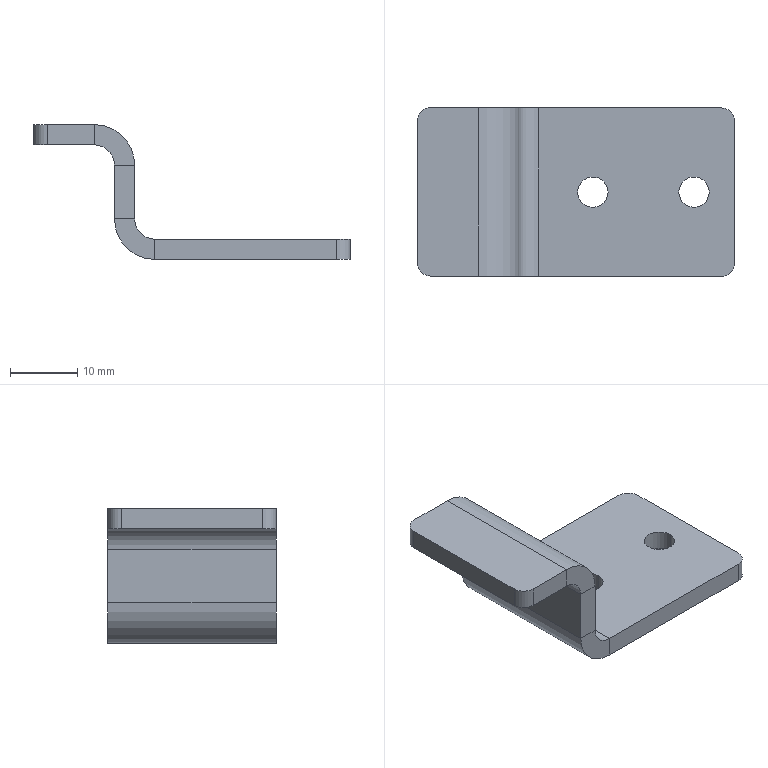Part | SolidWorks | features EdgeFlange 2, Fillet 1, FlatPattern 1, ICE 1, SMBaseFlange 1, SheetMetal 1 | 1 solid | 30 faces | box 47 x 25 x 20 mm | volume 4405 mm3 | plane 18 | cylinder 12 | commonest cylinder face diameters 4 x4 4.5 x4 6 x2 12 x2
STEP:
#1=CARTESIAN_POINT('',(-5.75,0.,-3.));
#2=VERTEX_POINT('',#1);
#3=CARTESIAN_POINT('',(-1.25,0.,-3.));
#4=VERTEX_POINT('',#3);
#5=CARTESIAN_POINT('',(-3.5,0.,-3.));
#6=DIRECTION('',(0.,0.,1.));
#7=DIRECTION('',(1.,0.,0.));
#8=AXIS2_PLACEMENT_3D('',#5,#6,#7);
#9=CIRCLE('',#8,2.25);
#10=EDGE_CURVE('',#2,#4,#9,.T.);
#11=ORIENTED_EDGE('',*,*,#10,.F.);
#12=CARTESIAN_POINT('',(-5.75,0.,0.));
#13=VERTEX_POINT('',#12);
#14=CARTESIAN_POINT('',(-5.75,0.,-3.));
#15=DIRECTION('',(0.,0.,1.));
#16=VECTOR('',#15,1000.);
#17=LINE('',#14,#16);
#18=EDGE_CURVE('',#2,#13,#17,.T.);
#19=ORIENTED_EDGE('',*,*,#18,.T.);
#20=CARTESIAN_POINT('',(-1.25,0.,0.));
#21=VERTEX_POINT('',#20);
#22=CARTESIAN_POINT('',(-3.5,0.,0.));
#23=DIRECTION('',(0.,0.,1.));
#24=DIRECTION('',(1.,0.,0.));
#25=AXIS2_PLACEMENT_3D('',#22,#23,#24);
#26=CIRCLE('',#25,2.25);
#27=EDGE_CURVE('',#13,#21,#26,.T.);
#28=ORIENTED_EDGE('',*,*,#27,.T.);
#29=CARTESIAN_POINT('',(-1.25,0.,-3.));
#30=DIRECTION('',(0.,0.,1.));
#31=VECTOR('',#30,1000.);
#32=LINE('',#29,#31);
#33=EDGE_CURVE('',#4,#21,#32,.T.);
#34=ORIENTED_EDGE('',*,*,#33,.F.);
#35=EDGE_LOOP('',(#11,#19,#28,#34));
#36=FACE_OUTER_BOUND('',#35,.T.);
#37=CARTESIAN_POINT('',(-3.5,0.,-3.));
#38=DIRECTION('',(0.,0.,1.));
#39=DIRECTION('',(1.,0.,0.));
#40=AXIS2_PLACEMENT_3D('',#37,#38,#39);
#41=CYLINDRICAL_SURFACE('',#40,2.25);
#42=ADVANCED_FACE('',(#36),#41,.F.);
#43=CARTESIAN_POINT('',(9.25,0.,-3.));
#44=VERTEX_POINT('',#43);
#45=CARTESIAN_POINT('',(13.75,0.,-3.));
#46=VERTEX_POINT('',#45);
#47=CARTESIAN_POINT('',(11.5,0.,-3.));
#48=DIRECTION('',(0.,0.,1.));
#49=DIRECTION('',(1.,0.,0.));
#50=AXIS2_PLACEMENT_3D('',#47,#48,#49);
#51=CIRCLE('',#50,2.25);
#52=EDGE_CURVE('',#44,#46,#51,.T.);
#53=ORIENTED_EDGE('',*,*,#52,.F.);
#54=CARTESIAN_POINT('',(9.25,0.,0.));
#55=VERTEX_POINT('',#54);
#56=CARTESIAN_POINT('',(9.25,0.,-3.));
#57=DIRECTION('',(0.,0.,1.));
#58=VECTOR('',#57,1000.);
#59=LINE('',#56,#58);
#60=EDGE_CURVE('',#44,#55,#59,.T.);
#61=ORIENTED_EDGE('',*,*,#60,.T.);
#62=CARTESIAN_POINT('',(13.75,0.,0.));
#63=VERTEX_POINT('',#62);
#64=CARTESIAN_POINT('',(11.5,0.,0.));
#65=DIRECTION('',(0.,0.,1.));
#66=DIRECTION('',(1.,0.,0.));
#67=AXIS2_PLACEMENT_3D('',#64,#65,#66);
#68=CIRCLE('',#67,2.25);
#69=EDGE_CURVE('',#55,#63,#68,.T.);
#70=ORIENTED_EDGE('',*,*,#69,.T.);
#71=CARTESIAN_POINT('',(13.75,0.,-3.));
#72=DIRECTION('',(0.,0.,1.));
#73=VECTOR('',#72,1000.);
#74=LINE('',#71,#73);
#75=EDGE_CURVE('',#46,#63,#74,.T.);
#76=ORIENTED_EDGE('',*,*,#75,.F.);
#77=EDGE_LOOP('',(#53,#61,#70,#76));
#78=FACE_OUTER_BOUND('',#77,.T.);
#79=CARTESIAN_POINT('',(11.5,0.,-3.));
#80=DIRECTION('',(0.,0.,1.));
#81=DIRECTION('',(1.,0.,0.));
#82=AXIS2_PLACEMENT_3D('',#79,#80,#81);
#83=CYLINDRICAL_SURFACE('',#82,2.25);
#84=ADVANCED_FACE('',(#78),#83,.F.);
#85=CARTESIAN_POINT('',(-17.5,12.5,3.));
#86=VERTEX_POINT('',#85);
#87=CARTESIAN_POINT('',(-17.5,12.5,11.));
#88=VERTEX_POINT('',#87);
#89=CARTESIAN_POINT('',(-17.5,12.5,17.));
#90=DIRECTION('',(0.,0.,1.));
#91=VECTOR('',#90,1000.);
#92=LINE('',#89,#91);
#93=EDGE_CURVE('',#86,#88,#92,.T.);
#94=ORIENTED_EDGE('',*,*,#93,.T.);
#95=CARTESIAN_POINT('',(-14.5,12.5,11.));
#96=VERTEX_POINT('',#95);
#97=CARTESIAN_POINT('',(-17.5,12.5,11.));
#98=DIRECTION('',(1.,0.,0.));
#99=VECTOR('',#98,1000.);
#100=LINE('',#97,#99);
#101=EDGE_CURVE('',#88,#96,#100,.T.);
#102=ORIENTED_EDGE('',*,*,#101,.T.);
#103=CARTESIAN_POINT('',(-14.5,12.5,3.));
#104=VERTEX_POINT('',#103);
#105=CARTESIAN_POINT('',(-14.5,12.5,0.));
#106=DIRECTION('',(0.,0.,1.));
#107=VECTOR('',#106,1000.);
#108=LINE('',#105,#107);
#109=EDGE_CURVE('',#104,#96,#108,.T.);
#110=ORIENTED_EDGE('',*,*,#109,.F.);
#111=CARTESIAN_POINT('',(-17.5,12.5,3.));
#112=DIRECTION('',(-1.,0.,0.));
#113=VECTOR('',#112,1000.);
#114=LINE('',#111,#113);
#115=EDGE_CURVE('',#104,#86,#114,.T.);
#116=ORIENTED_EDGE('',*,*,#115,.T.);
#117=EDGE_LOOP('',(#94,#102,#110,#116));
#118=FACE_OUTER_BOUND('',#117,.T.);
#119=CARTESIAN_POINT('',(-17.5,12.5,17.));
#120=DIRECTION('',(0.,1.,0.));
#121=DIRECTION('',(0.,0.,1.));
#122=AXIS2_PLACEMENT_3D('',#119,#120,#121);
#123=PLANE('',#122);
#124=ADVANCED_FACE('',(#118),#123,.T.);
#125=CARTESIAN_POINT('',(-17.5,-12.5,11.));
#126=VERTEX_POINT('',#125);
#127=CARTESIAN_POINT('',(-17.5,-12.5,3.));
#128=VERTEX_POINT('',#127);
#129=CARTESIAN_POINT('',(-17.5,-12.5,0.));
#130=DIRECTION('',(0.,0.,-1.));
#131=VECTOR('',#130,1000.);
#132=LINE('',#129,#131);
#133=EDGE_CURVE('',#126,#128,#132,.T.);
#134=ORIENTED_EDGE('',*,*,#133,.F.);
#135=CARTESIAN_POINT('',(-17.5,12.5,11.));
#136=DIRECTION('',(0.,-1.,0.));
#137=VECTOR('',#136,1000.);
#138=LINE('',#135,#137);
#139=EDGE_CURVE('',#88,#126,#138,.T.);
#140=ORIENTED_EDGE('',*,*,#139,.F.);
#141=ORIENTED_EDGE('',*,*,#93,.F.);
#142=CARTESIAN_POINT('',(-17.5,0.,3.));
#143=DIRECTION('',(0.,-1.,0.));
#144=VECTOR('',#143,1000.);
#145=LINE('',#142,#144);
#146=EDGE_CURVE('',#86,#128,#145,.T.);
#147=ORIENTED_EDGE('',*,*,#146,.T.);
#148=EDGE_LOOP('',(#134,#140,#141,#147));
#149=FACE_OUTER_BOUND('',#148,.T.);
#150=CARTESIAN_POINT('',(-17.5,0.,0.));
#151=DIRECTION('',(-1.,0.,0.));
#152=DIRECTION('',(0.,0.,1.));
#153=AXIS2_PLACEMENT_3D('',#150,#151,#152);
#154=PLANE('',#153);
#155=ADVANCED_FACE('',(#149),#154,.T.);
#156=CARTESIAN_POINT('',(-14.5,-12.5,11.));
#157=VERTEX_POINT('',#156);
#158=CARTESIAN_POINT('',(-14.5,12.5,11.));
#159=DIRECTION('',(0.,-1.,0.));
#160=VECTOR('',#159,1000.);
#161=LINE('',#158,#160);
#162=EDGE_CURVE('',#96,#157,#161,.T.);
#163=ORIENTED_EDGE('',*,*,#162,.T.);
#164=CARTESIAN_POINT('',(-14.5,-12.5,3.));
#165=VERTEX_POINT('',#164);
#166=CARTESIAN_POINT('',(-14.5,-12.5,0.));
#167=DIRECTION('',(0.,0.,-1.));
#168=VECTOR('',#167,1000.);
#169=LINE('',#166,#168);
#170=EDGE_CURVE('',#157,#165,#169,.T.);
#171=ORIENTED_EDGE('',*,*,#170,.T.);
#172=CARTESIAN_POINT('',(-14.5,12.5,3.));
#173=DIRECTION('',(0.,-1.,0.));
#174=VECTOR('',#173,1000.);
#175=LINE('',#172,#174);
#176=EDGE_CURVE('',#104,#165,#175,.T.);
#177=ORIENTED_EDGE('',*,*,#176,.F.);
#178=ORIENTED_EDGE('',*,*,#109,.T.);
#179=EDGE_LOOP('',(#163,#171,#177,#178));
#180=FACE_OUTER_BOUND('',#179,.T.);
#181=CARTESIAN_POINT('',(-14.5,0.,0.));
#182=DIRECTION('',(-1.,0.,0.));
#183=DIRECTION('',(0.,0.,1.));
#184=AXIS2_PLACEMENT_3D('',#181,#182,#183);
#185=PLANE('',#184);
#186=ADVANCED_FACE('',(#180),#185,.F.);
#187=CARTESIAN_POINT('',(-11.5,-12.5,-3.));
#188=VERTEX_POINT('',#187);
#189=CARTESIAN_POINT('',(15.5,-12.5,-3.));
#190=VERTEX_POINT('',#189);
#191=CARTESIAN_POINT('',(-17.5,-12.5,-3.));
#192=DIRECTION('',(1.,0.,0.));
#193=VECTOR('',#192,1000.);
#194=LINE('',#191,#193);
#195=EDGE_CURVE('',#188,#190,#194,.T.);
#196=ORIENTED_EDGE('',*,*,#195,.T.);
#197=CARTESIAN_POINT('',(15.5,-12.5,0.));
#198=VERTEX_POINT('',#197);
#199=CARTESIAN_POINT('',(15.5,-12.5,-3.));
#200=DIRECTION('',(0.,0.,1.));
#201=VECTOR('',#200,1000.);
#202=LINE('',#199,#201);
#203=EDGE_CURVE('',#190,#198,#202,.T.);
#204=ORIENTED_EDGE('',*,*,#203,.T.);
#205=CARTESIAN_POINT('',(-11.5,-12.5,0.));
#206=VERTEX_POINT('',#205);
#207=CARTESIAN_POINT('',(-17.5,-12.5,0.));
#208=DIRECTION('',(1.,0.,0.));
#209=VECTOR('',#208,1000.);
#210=LINE('',#207,#209);
#211=EDGE_CURVE('',#206,#198,#210,.T.);
#212=ORIENTED_EDGE('',*,*,#211,.F.);
#213=CARTESIAN_POINT('',(-11.5,-12.5,0.));
#214=DIRECTION('',(0.,0.,-1.));
#215=VECTOR('',#214,1000.);
#216=LINE('',#213,#215);
#217=EDGE_CURVE('',#206,#188,#216,.T.);
#218=ORIENTED_EDGE('',*,*,#217,.T.);
#219=EDGE_LOOP('',(#196,#204,#212,#218));
#220=FACE_OUTER_BOUND('',#219,.T.);
#221=CARTESIAN_POINT('',(-17.5,-12.5,-3.));
#222=DIRECTION('',(0.,-1.,0.));
#223=DIRECTION('',(0.,0.,-1.));
#224=AXIS2_PLACEMENT_3D('',#221,#222,#223);
#225=PLANE('',#224);
#226=ADVANCED_FACE('',(#220),#225,.T.);
#227=CARTESIAN_POINT('',(-3.5,0.,-3.));
#228=DIRECTION('',(0.,0.,1.));
#229=DIRECTION('',(1.,0.,0.));
#230=AXIS2_PLACEMENT_3D('',#227,#228,#229);
#231=CIRCLE('',#230,2.25);
#232=EDGE_CURVE('',#4,#2,#231,.T.);
#233=ORIENTED_EDGE('',*,*,#232,.T.);
#234=ORIENTED_EDGE('',*,*,#10,.T.);
#235=EDGE_LOOP('',(#233,#234));
#236=FACE_BOUND('',#235,.T.);
#237=CARTESIAN_POINT('',(11.5,0.,-3.));
#238=DIRECTION('',(0.,0.,1.));
#239=DIRECTION('',(1.,0.,0.));
#240=AXIS2_PLACEMENT_3D('',#237,#238,#239);
#241=CIRCLE('',#240,2.25);
#242=EDGE_CURVE('',#46,#44,#241,.T.);
#243=ORIENTED_EDGE('',*,*,#242,.T.);
#244=ORIENTED_EDGE('',*,*,#52,.T.);
#245=EDGE_LOOP('',(#243,#244));
#246=FACE_BOUND('',#245,.T.);
#247=CARTESIAN_POINT('',(17.5,-10.5,-3.));
#248=VERTEX_POINT('',#247);
#249=CARTESIAN_POINT('',(17.5,10.5,-3.));
#250=VERTEX_POINT('',#249);
#251=CARTESIAN_POINT('',(17.5,12.5,-3.));
#252=DIRECTION('',(0.,1.,0.));
#253=VECTOR('',#252,1000.);
#254=LINE('',#251,#253);
#255=EDGE_CURVE('',#248,#250,#254,.T.);
#256=ORIENTED_EDGE('',*,*,#255,.F.);
#257=CARTESIAN_POINT('',(15.5,-10.5,-3.));
#258=DIRECTION('',(0.,0.,-1.));
#259=DIRECTION('',(1.,0.,0.));
#260=AXIS2_PLACEMENT_3D('',#257,#258,#259);
#261=CIRCLE('',#260,2.);
#262=EDGE_CURVE('',#248,#190,#261,.T.);
#263=ORIENTED_EDGE('',*,*,#262,.T.);
#264=ORIENTED_EDGE('',*,*,#195,.F.);
#265=CARTESIAN_POINT('',(-11.5,12.5,-3.));
#266=VERTEX_POINT('',#265);
#267=CARTESIAN_POINT('',(-11.5,-12.5,-3.));
#268=DIRECTION('',(0.,1.,0.));
#269=VECTOR('',#268,1000.);
#270=LINE('',#267,#269);
#271=EDGE_CURVE('',#188,#266,#270,.T.);
#272=ORIENTED_EDGE('',*,*,#271,.T.);
#273=CARTESIAN_POINT('',(15.5,12.5,-3.));
#274=VERTEX_POINT('',#273);
#275=CARTESIAN_POINT('',(-17.5,12.5,-3.));
#276=DIRECTION('',(-1.,0.,0.));
#277=VECTOR('',#276,1000.);
#278=LINE('',#275,#277);
#279=EDGE_CURVE('',#274,#266,#278,.T.);
#280=ORIENTED_EDGE('',*,*,#279,.F.);
#281=CARTESIAN_POINT('',(15.5,10.5,-3.));
#282=DIRECTION('',(0.,0.,-1.));
#283=DIRECTION('',(1.,0.,0.));
#284=AXIS2_PLACEMENT_3D('',#281,#282,#283);
#285=CIRCLE('',#284,2.);
#286=EDGE_CURVE('',#274,#250,#285,.T.);
#287=ORIENTED_EDGE('',*,*,#286,.T.);
#288=EDGE_LOOP('',(#256,#263,#264,#272,#280,#287));
#289=FACE_OUTER_BOUND('',#288,.T.);
#290=CARTESIAN_POINT('',(0.,0.,-3.));
#291=DIRECTION('',(0.,0.,1.));
#292=DIRECTION('',(1.,0.,0.));
#293=AXIS2_PLACEMENT_3D('',#290,#291,#292);
#294=PLANE('',#293);
#295=ADVANCED_FACE('',(#236,#246,#289),#294,.F.);
#296=CARTESIAN_POINT('',(-3.5,0.,0.));
#297=DIRECTION('',(0.,0.,1.));
#298=DIRECTION('',(1.,0.,0.));
#299=AXIS2_PLACEMENT_3D('',#296,#297,#298);
#300=CIRCLE('',#299,2.25);
#301=EDGE_CURVE('',#21,#13,#300,.T.);
#302=ORIENTED_EDGE('',*,*,#301,.F.);
#303=ORIENTED_EDGE('',*,*,#27,.F.);
#304=EDGE_LOOP('',(#302,#303));
#305=FACE_BOUND('',#304,.T.);
#306=CARTESIAN_POINT('',(11.5,0.,0.));
#307=DIRECTION('',(0.,0.,1.));
#308=DIRECTION('',(1.,0.,0.));
#309=AXIS2_PLACEMENT_3D('',#306,#307,#308);
#310=CIRCLE('',#309,2.25);
#311=EDGE_CURVE('',#63,#55,#310,.T.);
#312=ORIENTED_EDGE('',*,*,#311,.F.);
#313=ORIENTED_EDGE('',*,*,#69,.F.);
#314=EDGE_LOOP('',(#312,#313));
#315=FACE_BOUND('',#314,.T.);
#316=ORIENTED_EDGE('',*,*,#211,.T.);
#317=CARTESIAN_POINT('',(17.5,-10.5,0.));
#318=VERTEX_POINT('',#317);
#319=CARTESIAN_POINT('',(15.5,-10.5,0.));
#320=DIRECTION('',(0.,0.,1.));
#321=DIRECTION('',(1.,0.,0.));
#322=AXIS2_PLACEMENT_3D('',#319,#320,#321);
#323=CIRCLE('',#322,2.);
#324=EDGE_CURVE('',#198,#318,#323,.T.);
#325=ORIENTED_EDGE('',*,*,#324,.T.);
#326=CARTESIAN_POINT('',(17.5,10.5,0.));
#327=VERTEX_POINT('',#326);
#328=CARTESIAN_POINT('',(17.5,12.5,0.));
#329=DIRECTION('',(0.,1.,0.));
#330=VECTOR('',#329,1000.);
#331=LINE('',#328,#330);
#332=EDGE_CURVE('',#318,#327,#331,.T.);
#333=ORIENTED_EDGE('',*,*,#332,.T.);
#334=CARTESIAN_POINT('',(15.5,12.5,0.));
#335=VERTEX_POINT('',#334);
#336=CARTESIAN_POINT('',(15.5,10.5,0.));
#337=DIRECTION('',(0.,0.,1.));
#338=DIRECTION('',(1.,0.,0.));
#339=AXIS2_PLACEMENT_3D('',#336,#337,#338);
#340=CIRCLE('',#339,2.);
#341=EDGE_CURVE('',#327,#335,#340,.T.);
#342=ORIENTED_EDGE('',*,*,#341,.T.);
#343=CARTESIAN_POINT('',(-11.5,12.5,0.));
#344=VERTEX_POINT('',#343);
#345=CARTESIAN_POINT('',(-17.5,12.5,0.));
#346=DIRECTION('',(-1.,0.,0.));
#347=VECTOR('',#346,1000.);
#348=LINE('',#345,#347);
#349=EDGE_CURVE('',#335,#344,#348,.T.);
#350=ORIENTED_EDGE('',*,*,#349,.T.);
#351=CARTESIAN_POINT('',(-11.5,-12.5,0.));
#352=DIRECTION('',(0.,1.,0.));
#353=VECTOR('',#352,1000.);
#354=LINE('',#351,#353);
#355=EDGE_CURVE('',#206,#344,#354,.T.);
#356=ORIENTED_EDGE('',*,*,#355,.F.);
#357=EDGE_LOOP('',(#316,#325,#333,#342,#350,#356));
#358=FACE_OUTER_BOUND('',#357,.T.);
#359=CARTESIAN_POINT('',(0.,0.,0.));
#360=DIRECTION('',(0.,0.,1.));
#361=DIRECTION('',(1.,0.,0.));
#362=AXIS2_PLACEMENT_3D('',#359,#360,#361);
#363=PLANE('',#362);
#364=ADVANCED_FACE('',(#305,#315,#358),#363,.T.);
#365=ORIENTED_EDGE('',*,*,#332,.F.);
#366=CARTESIAN_POINT('',(17.5,-10.5,-3.));
#367=DIRECTION('',(0.,0.,-1.));
#368=VECTOR('',#367,1000.);
#369=LINE('',#366,#368);
#370=EDGE_CURVE('',#318,#248,#369,.T.);
#371=ORIENTED_EDGE('',*,*,#370,.T.);
#372=ORIENTED_EDGE('',*,*,#255,.T.);
#373=CARTESIAN_POINT('',(17.5,10.5,-3.));
#374=DIRECTION('',(0.,0.,1.));
#375=VECTOR('',#374,1000.);
#376=LINE('',#373,#375);
#377=EDGE_CURVE('',#250,#327,#376,.T.);
#378=ORIENTED_EDGE('',*,*,#377,.T.);
#379=EDGE_LOOP('',(#365,#371,#372,#378));
#380=FACE_OUTER_BOUND('',#379,.T.);
#381=CARTESIAN_POINT('',(17.5,12.5,-3.));
#382=DIRECTION('',(1.,0.,0.));
#383=DIRECTION('',(0.,0.,-1.));
#384=AXIS2_PLACEMENT_3D('',#381,#382,#383);
#385=PLANE('',#384);
#386=ADVANCED_FACE('',(#380),#385,.T.);
#387=ORIENTED_EDGE('',*,*,#349,.F.);
#388=CARTESIAN_POINT('',(15.5,12.5,-3.));
#389=DIRECTION('',(0.,0.,-1.));
#390=VECTOR('',#389,1000.);
#391=LINE('',#388,#390);
#392=EDGE_CURVE('',#335,#274,#391,.T.);
#393=ORIENTED_EDGE('',*,*,#392,.T.);
#394=ORIENTED_EDGE('',*,*,#279,.T.);
#395=CARTESIAN_POINT('',(-11.5,12.5,0.));
#396=DIRECTION('',(0.,0.,-1.));
#397=VECTOR('',#396,1000.);
#398=LINE('',#395,#397);
#399=EDGE_CURVE('',#344,#266,#398,.T.);
#400=ORIENTED_EDGE('',*,*,#399,.F.);
#401=EDGE_LOOP('',(#387,#393,#394,#400));
#402=FACE_OUTER_BOUND('',#401,.T.);
#403=CARTESIAN_POINT('',(-17.5,12.5,-3.));
#404=DIRECTION('',(0.,1.,0.));
#405=DIRECTION('',(0.,0.,1.));
#406=AXIS2_PLACEMENT_3D('',#403,#404,#405);
#407=PLANE('',#406);
#408=ADVANCED_FACE('',(#402),#407,.T.);
#409=ORIENTED_EDGE('',*,*,#115,.F.);
#410=CARTESIAN_POINT('',(-11.5,12.5,3.));
#411=DIRECTION('',(0.,1.,0.));
#412=DIRECTION('',(0.,0.,-1.));
#413=AXIS2_PLACEMENT_3D('',#410,#411,#412);
#414=CIRCLE('',#413,3.);
#415=EDGE_CURVE('',#344,#104,#414,.T.);
#416=ORIENTED_EDGE('',*,*,#415,.F.);
#417=ORIENTED_EDGE('',*,*,#399,.T.);
#418=CARTESIAN_POINT('',(-11.5,12.5,3.));
#419=DIRECTION('',(0.,1.,0.));
#420=DIRECTION('',(0.,0.,-1.));
#421=AXIS2_PLACEMENT_3D('',#418,#419,#420);
#422=CIRCLE('',#421,6.);
#423=EDGE_CURVE('',#266,#86,#422,.T.);
#424=ORIENTED_EDGE('',*,*,#423,.T.);
#425=EDGE_LOOP('',(#409,#416,#417,#424));
#426=FACE_OUTER_BOUND('',#425,.T.);
#427=CARTESIAN_POINT('',(-11.5,12.5,3.));
#428=DIRECTION('',(0.,1.,0.));
#429=DIRECTION('',(0.,0.,1.));
#430=AXIS2_PLACEMENT_3D('',#427,#428,#429);
#431=PLANE('',#430);
#432=ADVANCED_FACE('',(#426),#431,.T.);
#433=CARTESIAN_POINT('',(-11.5,-12.5,3.));
#434=DIRECTION('',(0.,-1.,0.));
#435=DIRECTION('',(0.,0.,-1.));
#436=AXIS2_PLACEMENT_3D('',#433,#434,#435);
#437=CIRCLE('',#436,3.);
#438=EDGE_CURVE('',#165,#206,#437,.T.);
#439=ORIENTED_EDGE('',*,*,#438,.F.);
#440=CARTESIAN_POINT('',(-14.5,-12.5,3.));
#441=DIRECTION('',(-1.,0.,0.));
#442=VECTOR('',#441,1000.);
#443=LINE('',#440,#442);
#444=EDGE_CURVE('',#165,#128,#443,.T.);
#445=ORIENTED_EDGE('',*,*,#444,.T.);
#446=CARTESIAN_POINT('',(-11.5,-12.5,3.));
#447=DIRECTION('',(0.,-1.,0.));
#448=DIRECTION('',(0.,0.,-1.));
#449=AXIS2_PLACEMENT_3D('',#446,#447,#448);
#450=CIRCLE('',#449,6.);
#451=EDGE_CURVE('',#128,#188,#450,.T.);
#452=ORIENTED_EDGE('',*,*,#451,.T.);
#453=ORIENTED_EDGE('',*,*,#217,.F.);
#454=EDGE_LOOP('',(#439,#445,#452,#453));
#455=FACE_OUTER_BOUND('',#454,.T.);
#456=CARTESIAN_POINT('',(-11.5,-12.5,3.));
#457=DIRECTION('',(0.,1.,0.));
#458=DIRECTION('',(0.,0.,1.));
#459=AXIS2_PLACEMENT_3D('',#456,#457,#458);
#460=PLANE('',#459);
#461=ADVANCED_FACE('',(#455),#460,.F.);
#462=ORIENTED_EDGE('',*,*,#271,.F.);
#463=ORIENTED_EDGE('',*,*,#451,.F.);
#464=ORIENTED_EDGE('',*,*,#146,.F.);
#465=ORIENTED_EDGE('',*,*,#423,.F.);
#466=EDGE_LOOP('',(#462,#463,#464,#465));
#467=FACE_OUTER_BOUND('',#466,.T.);
#468=CARTESIAN_POINT('',(-11.5,-12.5,3.));
#469=DIRECTION('',(0.,-1.,0.));
#470=DIRECTION('',(-1.,0.,0.));
#471=AXIS2_PLACEMENT_3D('',#468,#469,#470);
#472=CYLINDRICAL_SURFACE('',#471,6.);
#473=ADVANCED_FACE('',(#467),#472,.T.);
#474=ORIENTED_EDGE('',*,*,#355,.T.);
#475=ORIENTED_EDGE('',*,*,#415,.T.);
#476=ORIENTED_EDGE('',*,*,#176,.T.);
#477=ORIENTED_EDGE('',*,*,#438,.T.);
#478=EDGE_LOOP('',(#474,#475,#476,#477));
#479=FACE_OUTER_BOUND('',#478,.T.);
#480=CARTESIAN_POINT('',(-11.5,-12.5,3.));
#481=DIRECTION('',(0.,-1.,0.));
#482=DIRECTION('',(-1.,0.,0.));
#483=AXIS2_PLACEMENT_3D('',#480,#481,#482);
#484=CYLINDRICAL_SURFACE('',#483,3.);
#485=ADVANCED_FACE('',(#479),#484,.F.);
#486=CARTESIAN_POINT('',(-17.5,-12.5,11.));
#487=DIRECTION('',(1.,0.,0.));
#488=VECTOR('',#487,1000.);
#489=LINE('',#486,#488);
#490=EDGE_CURVE('',#126,#157,#489,.T.);
#491=ORIENTED_EDGE('',*,*,#490,.F.);
#492=ORIENTED_EDGE('',*,*,#133,.T.);
#493=ORIENTED_EDGE('',*,*,#444,.F.);
#494=ORIENTED_EDGE('',*,*,#170,.F.);
#495=EDGE_LOOP('',(#491,#492,#493,#494));
#496=FACE_OUTER_BOUND('',#495,.T.);
#497=CARTESIAN_POINT('',(-17.5,-12.5,0.));
#498=DIRECTION('',(0.,-1.,0.));
#499=DIRECTION('',(0.,0.,-1.));
#500=AXIS2_PLACEMENT_3D('',#497,#498,#499);
#501=PLANE('',#500);
#502=ADVANCED_FACE('',(#496),#501,.T.);
#503=CARTESIAN_POINT('',(-20.5,-12.5,14.));
#504=VERTEX_POINT('',#503);
#505=CARTESIAN_POINT('',(-20.5,-12.5,17.));
#506=VERTEX_POINT('',#505);
#507=CARTESIAN_POINT('',(-20.5,-12.5,17.));
#508=DIRECTION('',(0.,0.,1.));
#509=VECTOR('',#508,1000.);
#510=LINE('',#507,#509);
#511=EDGE_CURVE('',#504,#506,#510,.T.);
#512=ORIENTED_EDGE('',*,*,#511,.F.);
#513=CARTESIAN_POINT('',(-20.5,-12.5,11.));
#514=DIRECTION('',(0.,-1.,0.));
#515=DIRECTION('',(0.,0.,1.));
#516=AXIS2_PLACEMENT_3D('',#513,#514,#515);
#517=CIRCLE('',#516,3.);
#518=EDGE_CURVE('',#126,#504,#517,.T.);
#519=ORIENTED_EDGE('',*,*,#518,.F.);
#520=ORIENTED_EDGE('',*,*,#490,.T.);
#521=CARTESIAN_POINT('',(-20.5,-12.5,11.));
#522=DIRECTION('',(0.,-1.,0.));
#523=DIRECTION('',(0.,0.,1.));
#524=AXIS2_PLACEMENT_3D('',#521,#522,#523);
#525=CIRCLE('',#524,6.);
#526=EDGE_CURVE('',#157,#506,#525,.T.);
#527=ORIENTED_EDGE('',*,*,#526,.T.);
#528=EDGE_LOOP('',(#512,#519,#520,#527));
#529=FACE_OUTER_BOUND('',#528,.T.);
#530=CARTESIAN_POINT('',(-20.5,-12.5,11.));
#531=DIRECTION('',(0.,-1.,0.));
#532=DIRECTION('',(0.,0.,-1.));
#533=AXIS2_PLACEMENT_3D('',#530,#531,#532);
#534=PLANE('',#533);
#535=ADVANCED_FACE('',(#529),#534,.T.);
#536=CARTESIAN_POINT('',(-20.5,12.5,14.));
#537=VERTEX_POINT('',#536);
#538=CARTESIAN_POINT('',(-20.5,12.5,11.));
#539=DIRECTION('',(0.,1.,0.));
#540=DIRECTION('',(0.,0.,1.));
#541=AXIS2_PLACEMENT_3D('',#538,#539,#540);
#542=CIRCLE('',#541,3.);
#543=EDGE_CURVE('',#537,#88,#542,.T.);
#544=ORIENTED_EDGE('',*,*,#543,.F.);
#545=CARTESIAN_POINT('',(-20.5,12.5,17.));
#546=VERTEX_POINT('',#545);
#547=CARTESIAN_POINT('',(-20.5,12.5,14.));
#548=DIRECTION('',(0.,0.,1.));
#549=VECTOR('',#548,1000.);
#550=LINE('',#547,#549);
#551=EDGE_CURVE('',#537,#546,#550,.T.);
#552=ORIENTED_EDGE('',*,*,#551,.T.);
#553=CARTESIAN_POINT('',(-20.5,12.5,11.));
#554=DIRECTION('',(0.,1.,0.));
#555=DIRECTION('',(0.,0.,1.));
#556=AXIS2_PLACEMENT_3D('',#553,#554,#555);
#557=CIRCLE('',#556,6.);
#558=EDGE_CURVE('',#546,#96,#557,.T.);
#559=ORIENTED_EDGE('',*,*,#558,.T.);
#560=ORIENTED_EDGE('',*,*,#101,.F.);
#561=EDGE_LOOP('',(#544,#552,#559,#560));
#562=FACE_OUTER_BOUND('',#561,.T.);
#563=CARTESIAN_POINT('',(-20.5,12.5,11.));
#564=DIRECTION('',(0.,-1.,0.));
#565=DIRECTION('',(0.,0.,-1.));
#566=AXIS2_PLACEMENT_3D('',#563,#564,#565);
#567=PLANE('',#566);
#568=ADVANCED_FACE('',(#562),#567,.F.);
#569=ORIENTED_EDGE('',*,*,#162,.F.);
#570=ORIENTED_EDGE('',*,*,#558,.F.);
#571=CARTESIAN_POINT('',(-20.5,0.,17.));
#572=DIRECTION('',(0.,1.,0.));
#573=VECTOR('',#572,1000.);
#574=LINE('',#571,#573);
#575=EDGE_CURVE('',#506,#546,#574,.T.);
#576=ORIENTED_EDGE('',*,*,#575,.F.);
#577=ORIENTED_EDGE('',*,*,#526,.F.);
#578=EDGE_LOOP('',(#569,#570,#576,#577));
#579=FACE_OUTER_BOUND('',#578,.T.);
#580=CARTESIAN_POINT('',(-20.5,12.5,11.));
#581=DIRECTION('',(0.,1.,0.));
#582=DIRECTION('',(0.,0.,1.));
#583=AXIS2_PLACEMENT_3D('',#580,#581,#582);
#584=CYLINDRICAL_SURFACE('',#583,6.);
#585=ADVANCED_FACE('',(#579),#584,.T.);
#586=ORIENTED_EDGE('',*,*,#139,.T.);
#587=ORIENTED_EDGE('',*,*,#518,.T.);
#588=CARTESIAN_POINT('',(-20.5,-12.5,14.));
#589=DIRECTION('',(0.,1.,0.));
#590=VECTOR('',#589,1000.);
#591=LINE('',#588,#590);
#592=EDGE_CURVE('',#504,#537,#591,.T.);
#593=ORIENTED_EDGE('',*,*,#592,.T.);
#594=ORIENTED_EDGE('',*,*,#543,.T.);
#595=EDGE_LOOP('',(#586,#587,#593,#594));
#596=FACE_OUTER_BOUND('',#595,.T.);
#597=CARTESIAN_POINT('',(-20.5,12.5,11.));
#598=DIRECTION('',(0.,1.,0.));
#599=DIRECTION('',(0.,0.,1.));
#600=AXIS2_PLACEMENT_3D('',#597,#598,#599);
#601=CYLINDRICAL_SURFACE('',#600,3.);
#602=ADVANCED_FACE('',(#596),#601,.F.);
#603=CARTESIAN_POINT('',(-27.5,12.5,14.));
#604=VERTEX_POINT('',#603);
#605=CARTESIAN_POINT('',(0.,12.5,14.));
#606=DIRECTION('',(1.,0.,0.));
#607=VECTOR('',#606,1000.);
#608=LINE('',#605,#607);
#609=EDGE_CURVE('',#604,#537,#608,.T.);
#610=ORIENTED_EDGE('',*,*,#609,.F.);
#611=CARTESIAN_POINT('',(-27.5,12.5,17.));
#612=VERTEX_POINT('',#611);
#613=CARTESIAN_POINT('',(-27.5,12.5,17.));
#614=DIRECTION('',(0.,0.,1.));
#615=VECTOR('',#614,1000.);
#616=LINE('',#613,#615);
#617=EDGE_CURVE('',#604,#612,#616,.T.);
#618=ORIENTED_EDGE('',*,*,#617,.T.);
#619=CARTESIAN_POINT('',(-17.5,12.5,17.));
#620=DIRECTION('',(1.,0.,0.));
#621=VECTOR('',#620,1000.);
#622=LINE('',#619,#621);
#623=EDGE_CURVE('',#612,#546,#622,.T.);
#624=ORIENTED_EDGE('',*,*,#623,.T.);
#625=ORIENTED_EDGE('',*,*,#551,.F.);
#626=EDGE_LOOP('',(#610,#618,#624,#625));
#627=FACE_OUTER_BOUND('',#626,.T.);
#628=CARTESIAN_POINT('',(-17.5,12.5,17.));
#629=DIRECTION('',(0.,1.,0.));
#630=DIRECTION('',(0.,0.,1.));
#631=AXIS2_PLACEMENT_3D('',#628,#629,#630);
#632=PLANE('',#631);
#633=ADVANCED_FACE('',(#627),#632,.T.);
#634=CARTESIAN_POINT('',(-27.5,-12.5,17.));
#635=VERTEX_POINT('',#634);
#636=CARTESIAN_POINT('',(-29.5,-12.5,17.));
#637=DIRECTION('',(-1.,0.,0.));
#638=VECTOR('',#637,1000.);
#639=LINE('',#636,#638);
#640=EDGE_CURVE('',#506,#635,#639,.T.);
#641=ORIENTED_EDGE('',*,*,#640,.T.);
#642=CARTESIAN_POINT('',(-27.5,-12.5,14.));
#643=VERTEX_POINT('',#642);
#644=CARTESIAN_POINT('',(-27.5,-12.5,17.));
#645=DIRECTION('',(0.,0.,-1.));
#646=VECTOR('',#645,1000.);
#647=LINE('',#644,#646);
#648=EDGE_CURVE('',#635,#643,#647,.T.);
#649=ORIENTED_EDGE('',*,*,#648,.T.);
#650=CARTESIAN_POINT('',(0.,-12.5,14.));
#651=DIRECTION('',(-1.,0.,0.));
#652=VECTOR('',#651,1000.);
#653=LINE('',#650,#652);
#654=EDGE_CURVE('',#504,#643,#653,.T.);
#655=ORIENTED_EDGE('',*,*,#654,.F.);
#656=ORIENTED_EDGE('',*,*,#511,.T.);
#657=EDGE_LOOP('',(#641,#649,#655,#656));
#658=FACE_OUTER_BOUND('',#657,.T.);
#659=CARTESIAN_POINT('',(-29.5,-12.5,17.));
#660=DIRECTION('',(0.,-1.,0.));
#661=DIRECTION('',(1.,0.,0.));
#662=AXIS2_PLACEMENT_3D('',#659,#660,#661);
#663=PLANE('',#662);
#664=ADVANCED_FACE('',(#658),#663,.T.);
#665=CARTESIAN_POINT('',(-29.5,-10.5,17.));
#666=VERTEX_POINT('',#665);
#667=CARTESIAN_POINT('',(-29.5,10.5,17.));
#668=VERTEX_POINT('',#667);
#669=CARTESIAN_POINT('',(-29.5,12.5,17.));
#670=DIRECTION('',(0.,1.,0.));
#671=VECTOR('',#670,1000.);
#672=LINE('',#669,#671);
#673=EDGE_CURVE('',#666,#668,#672,.T.);
#674=ORIENTED_EDGE('',*,*,#673,.F.);
#675=CARTESIAN_POINT('',(-27.5,-10.5,17.));
#676=DIRECTION('',(0.,0.,1.));
#677=DIRECTION('',(1.,0.,0.));
#678=AXIS2_PLACEMENT_3D('',#675,#676,#677);
#679=CIRCLE('',#678,2.);
#680=EDGE_CURVE('',#666,#635,#679,.T.);
#681=ORIENTED_EDGE('',*,*,#680,.T.);
#682=ORIENTED_EDGE('',*,*,#640,.F.);
#683=ORIENTED_EDGE('',*,*,#575,.T.);
#684=ORIENTED_EDGE('',*,*,#623,.F.);
#685=CARTESIAN_POINT('',(-27.5,10.5,17.));
#686=DIRECTION('',(0.,0.,1.));
#687=DIRECTION('',(1.,0.,0.));
#688=AXIS2_PLACEMENT_3D('',#685,#686,#687);
#689=CIRCLE('',#688,2.);
#690=EDGE_CURVE('',#612,#668,#689,.T.);
#691=ORIENTED_EDGE('',*,*,#690,.T.);
#692=EDGE_LOOP('',(#674,#681,#682,#683,#684,#691));
#693=FACE_OUTER_BOUND('',#692,.T.);
#694=CARTESIAN_POINT('',(0.,0.,17.));
#695=DIRECTION('',(0.,0.,1.));
#696=DIRECTION('',(1.,0.,0.));
#697=AXIS2_PLACEMENT_3D('',#694,#695,#696);
#698=PLANE('',#697);
#699=ADVANCED_FACE('',(#693),#698,.T.);
#700=ORIENTED_EDGE('',*,*,#654,.T.);
#701=CARTESIAN_POINT('',(-29.5,-10.5,14.));
#702=VERTEX_POINT('',#701);
#703=CARTESIAN_POINT('',(-27.5,-10.5,14.));
#704=DIRECTION('',(0.,0.,-1.));
#705=DIRECTION('',(1.,0.,0.));
#706=AXIS2_PLACEMENT_3D('',#703,#704,#705);
#707=CIRCLE('',#706,2.);
#708=EDGE_CURVE('',#643,#702,#707,.T.);
#709=ORIENTED_EDGE('',*,*,#708,.T.);
#710=CARTESIAN_POINT('',(-29.5,10.5,14.));
#711=VERTEX_POINT('',#710);
#712=CARTESIAN_POINT('',(-29.5,0.,14.));
#713=DIRECTION('',(0.,1.,0.));
#714=VECTOR('',#713,1000.);
#715=LINE('',#712,#714);
#716=EDGE_CURVE('',#702,#711,#715,.T.);
#717=ORIENTED_EDGE('',*,*,#716,.T.);
#718=CARTESIAN_POINT('',(-27.5,10.5,14.));
#719=DIRECTION('',(0.,0.,-1.));
#720=DIRECTION('',(1.,0.,0.));
#721=AXIS2_PLACEMENT_3D('',#718,#719,#720);
#722=CIRCLE('',#721,2.);
#723=EDGE_CURVE('',#711,#604,#722,.T.);
#724=ORIENTED_EDGE('',*,*,#723,.T.);
#725=ORIENTED_EDGE('',*,*,#609,.T.);
#726=ORIENTED_EDGE('',*,*,#592,.F.);
#727=EDGE_LOOP('',(#700,#709,#717,#724,#725,#726));
#728=FACE_OUTER_BOUND('',#727,.T.);
#729=CARTESIAN_POINT('',(0.,0.,14.));
#730=DIRECTION('',(0.,0.,1.));
#731=DIRECTION('',(1.,0.,0.));
#732=AXIS2_PLACEMENT_3D('',#729,#730,#731);
#733=PLANE('',#732);
#734=ADVANCED_FACE('',(#728),#733,.F.);
#735=ORIENTED_EDGE('',*,*,#716,.F.);
#736=CARTESIAN_POINT('',(-29.5,-10.5,17.));
#737=DIRECTION('',(0.,0.,1.));
#738=VECTOR('',#737,1000.);
#739=LINE('',#736,#738);
#740=EDGE_CURVE('',#702,#666,#739,.T.);
#741=ORIENTED_EDGE('',*,*,#740,.T.);
#742=ORIENTED_EDGE('',*,*,#673,.T.);
#743=CARTESIAN_POINT('',(-29.5,10.5,17.));
#744=DIRECTION('',(0.,0.,-1.));
#745=VECTOR('',#744,1000.);
#746=LINE('',#743,#745);
#747=EDGE_CURVE('',#668,#711,#746,.T.);
#748=ORIENTED_EDGE('',*,*,#747,.T.);
#749=EDGE_LOOP('',(#735,#741,#742,#748));
#750=FACE_OUTER_BOUND('',#749,.T.);
#751=CARTESIAN_POINT('',(-29.5,12.5,17.));
#752=DIRECTION('',(-1.,0.,0.));
#753=DIRECTION('',(0.,0.,1.));
#754=AXIS2_PLACEMENT_3D('',#751,#752,#753);
#755=PLANE('',#754);
#756=ADVANCED_FACE('',(#750),#755,.T.);
#757=ORIENTED_EDGE('',*,*,#262,.F.);
#758=ORIENTED_EDGE('',*,*,#370,.F.);
#759=ORIENTED_EDGE('',*,*,#324,.F.);
#760=ORIENTED_EDGE('',*,*,#203,.F.);
#761=EDGE_LOOP('',(#757,#758,#759,#760));
#762=FACE_OUTER_BOUND('',#761,.T.);
#763=CARTESIAN_POINT('',(15.5,-10.5,-3.));
#764=DIRECTION('',(0.,0.,1.));
#765=DIRECTION('',(1.,0.,0.));
#766=AXIS2_PLACEMENT_3D('',#763,#764,#765);
#767=CYLINDRICAL_SURFACE('',#766,2.);
#768=ADVANCED_FACE('',(#762),#767,.T.);
#769=ORIENTED_EDGE('',*,*,#286,.F.);
#770=ORIENTED_EDGE('',*,*,#392,.F.);
#771=ORIENTED_EDGE('',*,*,#341,.F.);
#772=ORIENTED_EDGE('',*,*,#377,.F.);
#773=EDGE_LOOP('',(#769,#770,#771,#772));
#774=FACE_OUTER_BOUND('',#773,.T.);
#775=CARTESIAN_POINT('',(15.5,10.5,-3.));
#776=DIRECTION('',(0.,0.,1.));
#777=DIRECTION('',(1.,0.,0.));
#778=AXIS2_PLACEMENT_3D('',#775,#776,#777);
#779=CYLINDRICAL_SURFACE('',#778,2.);
#780=ADVANCED_FACE('',(#774),#779,.T.);
#781=ORIENTED_EDGE('',*,*,#680,.F.);
#782=ORIENTED_EDGE('',*,*,#740,.F.);
#783=ORIENTED_EDGE('',*,*,#708,.F.);
#784=ORIENTED_EDGE('',*,*,#648,.F.);
#785=EDGE_LOOP('',(#781,#782,#783,#784));
#786=FACE_OUTER_BOUND('',#785,.T.);
#787=CARTESIAN_POINT('',(-27.5,-10.5,17.));
#788=DIRECTION('',(0.,0.,-1.));
#789=DIRECTION('',(-1.,0.,0.));
#790=AXIS2_PLACEMENT_3D('',#787,#788,#789);
#791=CYLINDRICAL_SURFACE('',#790,2.);
#792=ADVANCED_FACE('',(#786),#791,.T.);
#793=ORIENTED_EDGE('',*,*,#690,.F.);
#794=ORIENTED_EDGE('',*,*,#617,.F.);
#795=ORIENTED_EDGE('',*,*,#723,.F.);
#796=ORIENTED_EDGE('',*,*,#747,.F.);
#797=EDGE_LOOP('',(#793,#794,#795,#796));
#798=FACE_OUTER_BOUND('',#797,.T.);
#799=CARTESIAN_POINT('',(-27.5,10.5,17.));
#800=DIRECTION('',(0.,0.,-1.));
#801=DIRECTION('',(-1.,0.,0.));
#802=AXIS2_PLACEMENT_3D('',#799,#800,#801);
#803=CYLINDRICAL_SURFACE('',#802,2.);
#804=ADVANCED_FACE('',(#798),#803,.T.);
#805=ORIENTED_EDGE('',*,*,#60,.F.);
#806=ORIENTED_EDGE('',*,*,#242,.F.);
#807=ORIENTED_EDGE('',*,*,#75,.T.);
#808=ORIENTED_EDGE('',*,*,#311,.T.);
#809=EDGE_LOOP('',(#805,#806,#807,#808));
#810=FACE_OUTER_BOUND('',#809,.T.);
#811=CARTESIAN_POINT('',(11.5,0.,-3.));
#812=DIRECTION('',(0.,0.,1.));
#813=DIRECTION('',(1.,0.,0.));
#814=AXIS2_PLACEMENT_3D('',#811,#812,#813);
#815=CYLINDRICAL_SURFACE('',#814,2.25);
#816=ADVANCED_FACE('',(#810),#815,.F.);
#817=ORIENTED_EDGE('',*,*,#18,.F.);
#818=ORIENTED_EDGE('',*,*,#232,.F.);
#819=ORIENTED_EDGE('',*,*,#33,.T.);
#820=ORIENTED_EDGE('',*,*,#301,.T.);
#821=EDGE_LOOP('',(#817,#818,#819,#820));
#822=FACE_OUTER_BOUND('',#821,.T.);
#823=CARTESIAN_POINT('',(-3.5,0.,-3.));
#824=DIRECTION('',(0.,0.,1.));
#825=DIRECTION('',(1.,0.,0.));
#826=AXIS2_PLACEMENT_3D('',#823,#824,#825);
#827=CYLINDRICAL_SURFACE('',#826,2.25);
#828=ADVANCED_FACE('',(#822),#827,.F.);
#829=CLOSED_SHELL('',(#42,#84,#124,#155,#186,#226,#295,#364,#386,#408,#432,#461,#473,#485,#502,#535,#568,#585,#602,#633,#664,#699,#734,#756,#768,#780,#792,#804,#816,#828));
#830=MANIFOLD_SOLID_BREP('',#829);
#831=CARTESIAN_POINT('',(0.,0.,0.));
#832=DIRECTION('',(0.,0.,1.));
#833=DIRECTION('',(1.,0.,0.));
#834=AXIS2_PLACEMENT_3D('',#831,#832,#833);
#835=(LENGTH_UNIT()NAMED_UNIT(*)SI_UNIT(.MILLI.,.METRE.));
#836=UNCERTAINTY_MEASURE_WITH_UNIT(LENGTH_MEASURE(0.00001),#835,'','');
#837=(NAMED_UNIT(*)PLANE_ANGLE_UNIT()SI_UNIT($,.RADIAN.));
#838=(NAMED_UNIT(*)SI_UNIT($,.STERADIAN.)SOLID_ANGLE_UNIT());
#839=(GEOMETRIC_REPRESENTATION_CONTEXT(3)GLOBAL_UNCERTAINTY_ASSIGNED_CONTEXT((#836))GLOBAL_UNIT_ASSIGNED_CONTEXT((#835,#837,#838))REPRESENTATION_CONTEXT('',''));
#840=ADVANCED_BREP_SHAPE_REPRESENTATION('',(#830,#834),#839);